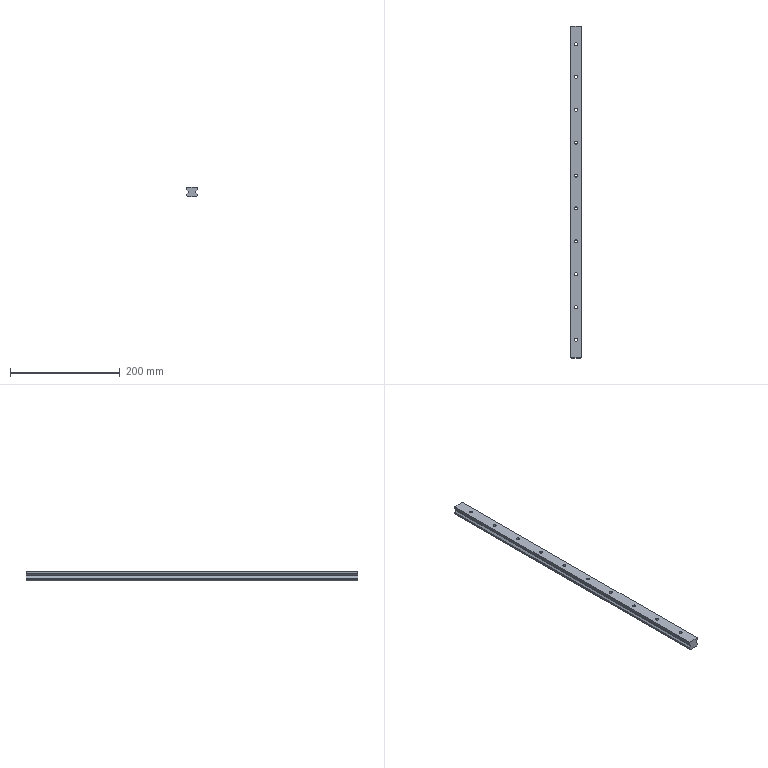Part | STEP file | HGW20CC guide rail-x1 | 1 solid | 66 faces | box 20 x 606 x 17.5 mm | volume 184749 mm3 | cylinder 40 | plane 26 | commonest cylinder face diameters 5.5 x20 10 x20